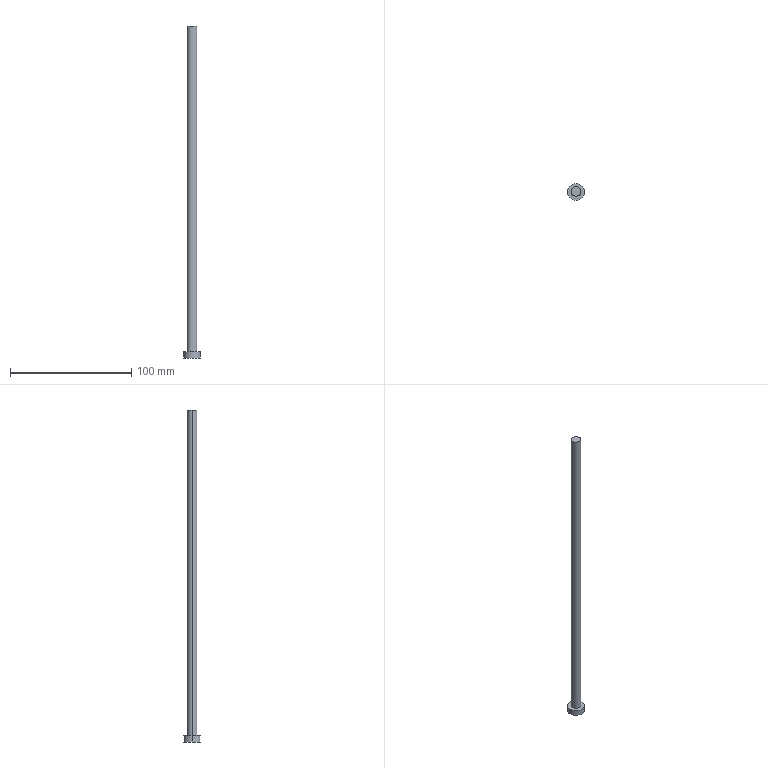Part | Creo | 1 solid | 7 faces | box 14 x 14 x 273.661 mm | volume 14274 mm3 | cylinder 4 | plane 3 | commonest cylinder face diameters 8 x2 14 x2
STEP:
#1=CARTESIAN_POINT('',(-56.147,-173.569,38.161));
#2=VERTEX_POINT('',#1);
#3=CARTESIAN_POINT('',(-64.147,-173.569,38.161));
#4=VERTEX_POINT('',#3);
#5=CARTESIAN_POINT('',(-60.147,-173.569,38.161));
#6=DIRECTION('',(0.,0.,1.));
#7=DIRECTION('',(1.,0.,0.));
#8=AXIS2_PLACEMENT_3D('',#5,#6,#7);
#9=CIRCLE('',#8,4.);
#10=EDGE_CURVE('',#2,#4,#9,.T.);
#11=ORIENTED_EDGE('',*,*,#10,.T.);
#12=CARTESIAN_POINT('',(-64.147,-173.569,-230.5));
#13=VERTEX_POINT('',#12);
#14=CARTESIAN_POINT('',(-64.147,-173.569,38.161));
#15=DIRECTION('',(0.,0.,-1.));
#16=VECTOR('',#15,268.661);
#17=LINE('',#14,#16);
#18=EDGE_CURVE('',#4,#13,#17,.T.);
#19=ORIENTED_EDGE('',*,*,#18,.T.);
#20=CARTESIAN_POINT('',(-56.147,-173.569,-230.5));
#21=VERTEX_POINT('',#20);
#22=CARTESIAN_POINT('',(-60.147,-173.569,-230.5));
#23=DIRECTION('',(0.,0.,-1.));
#24=DIRECTION('',(-1.,0.,0.));
#25=AXIS2_PLACEMENT_3D('',#22,#23,#24);
#26=CIRCLE('',#25,4.);
#27=EDGE_CURVE('',#13,#21,#26,.T.);
#28=ORIENTED_EDGE('',*,*,#27,.T.);
#29=CARTESIAN_POINT('',(-56.147,-173.569,38.161));
#30=DIRECTION('',(0.,0.,-1.));
#31=VECTOR('',#30,268.661);
#32=LINE('',#29,#31);
#33=EDGE_CURVE('',#2,#21,#32,.T.);
#34=ORIENTED_EDGE('',*,*,#33,.F.);
#35=EDGE_LOOP('',(#11,#19,#28,#34));
#36=FACE_OUTER_BOUND('',#35,.F.);
#37=CARTESIAN_POINT('',(-60.147,-173.569,49.5));
#38=DIRECTION('',(0.,0.,-1.));
#39=DIRECTION('',(-1.,0.,0.));
#40=AXIS2_PLACEMENT_3D('',#37,#38,#39);
#41=CYLINDRICAL_SURFACE('',#40,4.);
#42=ADVANCED_FACE('',(#36),#41,.T.);
#43=CARTESIAN_POINT('',(-60.147,-173.569,38.161));
#44=DIRECTION('',(0.,0.,1.));
#45=DIRECTION('',(-1.,0.,0.));
#46=AXIS2_PLACEMENT_3D('',#43,#44,#45);
#47=CIRCLE('',#46,4.);
#48=EDGE_CURVE('',#4,#2,#47,.T.);
#49=ORIENTED_EDGE('',*,*,#48,.F.);
#50=ORIENTED_EDGE('',*,*,#10,.F.);
#51=EDGE_LOOP('',(#49,#50));
#52=FACE_OUTER_BOUND('',#51,.F.);
#53=CARTESIAN_POINT('',(0.,0.,38.161));
#54=DIRECTION('',(0.,0.,-1.));
#55=DIRECTION('',(0.,1.,0.));
#56=AXIS2_PLACEMENT_3D('',#53,#54,#55);
#57=PLANE('',#56);
#58=ADVANCED_FACE('',(#52),#57,.F.);
#59=ORIENTED_EDGE('',*,*,#48,.T.);
#60=ORIENTED_EDGE('',*,*,#33,.T.);
#61=CARTESIAN_POINT('',(-60.147,-173.569,-230.5));
#62=DIRECTION('',(0.,0.,-1.));
#63=DIRECTION('',(1.,0.,0.));
#64=AXIS2_PLACEMENT_3D('',#61,#62,#63);
#65=CIRCLE('',#64,4.);
#66=EDGE_CURVE('',#21,#13,#65,.T.);
#67=ORIENTED_EDGE('',*,*,#66,.T.);
#68=ORIENTED_EDGE('',*,*,#18,.F.);
#69=EDGE_LOOP('',(#59,#60,#67,#68));
#70=FACE_OUTER_BOUND('',#69,.F.);
#71=CARTESIAN_POINT('',(-60.147,-173.569,49.5));
#72=DIRECTION('',(0.,0.,-1.));
#73=DIRECTION('',(-1.,0.,0.));
#74=AXIS2_PLACEMENT_3D('',#71,#72,#73);
#75=CYLINDRICAL_SURFACE('',#74,4.);
#76=ADVANCED_FACE('',(#70),#75,.T.);
#77=CARTESIAN_POINT('',(-67.147,-173.569,-230.5));
#78=VERTEX_POINT('',#77);
#79=CARTESIAN_POINT('',(-53.147,-173.569,-230.5));
#80=VERTEX_POINT('',#79);
#81=CARTESIAN_POINT('',(-60.147,-173.569,-230.5));
#82=DIRECTION('',(0.,0.,1.));
#83=DIRECTION('',(-1.,0.,0.));
#84=AXIS2_PLACEMENT_3D('',#81,#82,#83);
#85=CIRCLE('',#84,7.);
#86=EDGE_CURVE('',#78,#80,#85,.T.);
#87=ORIENTED_EDGE('',*,*,#86,.F.);
#88=CARTESIAN_POINT('',(-60.147,-173.569,-230.5));
#89=DIRECTION('',(0.,0.,1.));
#90=DIRECTION('',(1.,0.,0.));
#91=AXIS2_PLACEMENT_3D('',#88,#89,#90);
#92=CIRCLE('',#91,7.);
#93=EDGE_CURVE('',#80,#78,#92,.T.);
#94=ORIENTED_EDGE('',*,*,#93,.F.);
#95=EDGE_LOOP('',(#87,#94));
#96=FACE_OUTER_BOUND('',#95,.F.);
#97=ORIENTED_EDGE('',*,*,#27,.F.);
#98=ORIENTED_EDGE('',*,*,#66,.F.);
#99=EDGE_LOOP('',(#97,#98));
#100=FACE_BOUND('',#99,.F.);
#101=CARTESIAN_POINT('',(-60.147,-173.569,-230.5));
#102=DIRECTION('',(0.,0.,-1.));
#103=DIRECTION('',(-1.,0.,0.));
#104=AXIS2_PLACEMENT_3D('',#101,#102,#103);
#105=PLANE('',#104);
#106=ADVANCED_FACE('',(#96,#100),#105,.F.);
#107=CARTESIAN_POINT('',(-53.147,-173.569,-235.5));
#108=VERTEX_POINT('',#107);
#109=CARTESIAN_POINT('',(-67.147,-173.569,-235.5));
#110=VERTEX_POINT('',#109);
#111=CARTESIAN_POINT('',(-60.147,-173.569,-235.5));
#112=DIRECTION('',(0.,0.,-1.));
#113=DIRECTION('',(1.,0.,0.));
#114=AXIS2_PLACEMENT_3D('',#111,#112,#113);
#115=CIRCLE('',#114,7.);
#116=EDGE_CURVE('',#108,#110,#115,.T.);
#117=ORIENTED_EDGE('',*,*,#116,.T.);
#118=CARTESIAN_POINT('',(-67.147,-173.569,-230.5));
#119=DIRECTION('',(0.,0.,-1.));
#120=VECTOR('',#119,5.);
#121=LINE('',#118,#120);
#122=EDGE_CURVE('',#78,#110,#121,.T.);
#123=ORIENTED_EDGE('',*,*,#122,.F.);
#124=ORIENTED_EDGE('',*,*,#86,.T.);
#125=CARTESIAN_POINT('',(-53.147,-173.569,-230.5));
#126=DIRECTION('',(0.,0.,-1.));
#127=VECTOR('',#126,5.);
#128=LINE('',#125,#127);
#129=EDGE_CURVE('',#80,#108,#128,.T.);
#130=ORIENTED_EDGE('',*,*,#129,.T.);
#131=EDGE_LOOP('',(#117,#123,#124,#130));
#132=FACE_OUTER_BOUND('',#131,.F.);
#133=CARTESIAN_POINT('',(-60.147,-173.569,-245.913));
#134=DIRECTION('',(0.,0.,-1.));
#135=DIRECTION('',(-1.,0.,0.));
#136=AXIS2_PLACEMENT_3D('',#133,#134,#135);
#137=CYLINDRICAL_SURFACE('',#136,7.);
#138=ADVANCED_FACE('',(#132),#137,.T.);
#139=CARTESIAN_POINT('',(-60.147,-173.569,-235.5));
#140=DIRECTION('',(0.,0.,-1.));
#141=DIRECTION('',(-1.,0.,0.));
#142=AXIS2_PLACEMENT_3D('',#139,#140,#141);
#143=CIRCLE('',#142,7.);
#144=EDGE_CURVE('',#110,#108,#143,.T.);
#145=ORIENTED_EDGE('',*,*,#144,.F.);
#146=ORIENTED_EDGE('',*,*,#116,.F.);
#147=EDGE_LOOP('',(#145,#146));
#148=FACE_OUTER_BOUND('',#147,.F.);
#149=CARTESIAN_POINT('',(-56.147,-173.569,-235.5));
#150=DIRECTION('',(0.,0.,1.));
#151=DIRECTION('',(1.,0.,0.));
#152=AXIS2_PLACEMENT_3D('',#149,#150,#151);
#153=PLANE('',#152);
#154=ADVANCED_FACE('',(#148),#153,.F.);
#155=ORIENTED_EDGE('',*,*,#144,.T.);
#156=ORIENTED_EDGE('',*,*,#129,.F.);
#157=ORIENTED_EDGE('',*,*,#93,.T.);
#158=ORIENTED_EDGE('',*,*,#122,.T.);
#159=EDGE_LOOP('',(#155,#156,#157,#158));
#160=FACE_OUTER_BOUND('',#159,.F.);
#161=CARTESIAN_POINT('',(-60.147,-173.569,-245.913));
#162=DIRECTION('',(0.,0.,-1.));
#163=DIRECTION('',(-1.,0.,0.));
#164=AXIS2_PLACEMENT_3D('',#161,#162,#163);
#165=CYLINDRICAL_SURFACE('',#164,7.);
#166=ADVANCED_FACE('',(#160),#165,.T.);
#167=CLOSED_SHELL('',(#42,#58,#76,#106,#138,#154,#166));
#168=MANIFOLD_SOLID_BREP('',#167);
#169=(LENGTH_UNIT()NAMED_UNIT(*)SI_UNIT(.MILLI.,.METRE.));
#170=UNCERTAINTY_MEASURE_WITH_UNIT(LENGTH_MEASURE(0.02744),#169,'','');
#171=(NAMED_UNIT(*)PLANE_ANGLE_UNIT()SI_UNIT($,.RADIAN.));
#172=PLANE_ANGLE_MEASURE_WITH_UNIT(PLANE_ANGLE_MEASURE(0.01745),#171);
#173=(CONVERSION_BASED_UNIT('DEGREE',#172)NAMED_UNIT(*)PLANE_ANGLE_UNIT());
#174=(NAMED_UNIT(*)SI_UNIT($,.STERADIAN.)SOLID_ANGLE_UNIT());
#175=(GEOMETRIC_REPRESENTATION_CONTEXT(3)GLOBAL_UNCERTAINTY_ASSIGNED_CONTEXT((#170))GLOBAL_UNIT_ASSIGNED_CONTEXT((#169,#173,#174))REPRESENTATION_CONTEXT('',''));
#176=ADVANCED_BREP_SHAPE_REPRESENTATION('',(#168),#175);